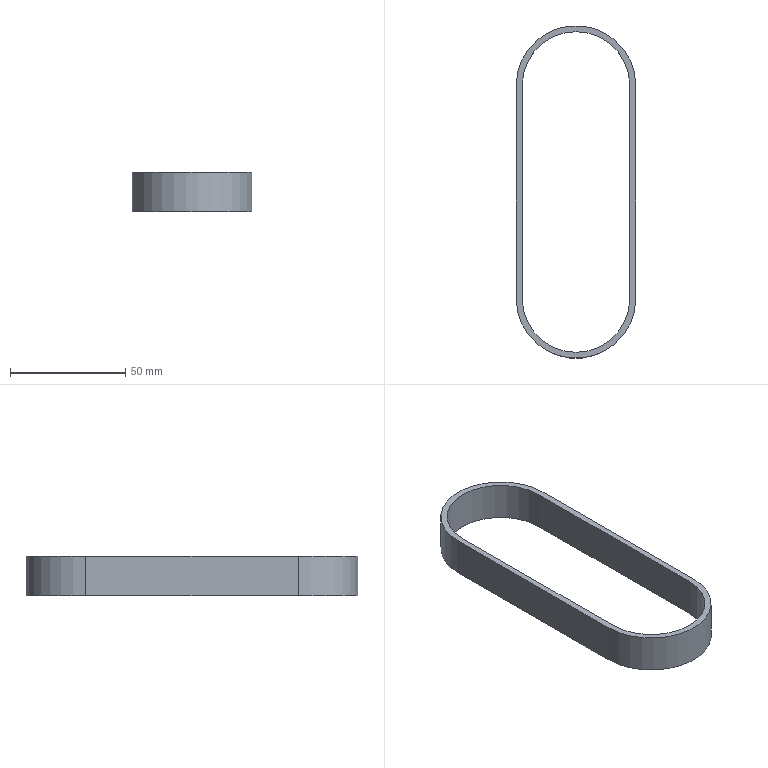Part | NX | features BREP 1 | 1 solid | 10 faces | box 52 x 144.5 x 17 mm | volume 15065 mm3 | plane 6 | cylinder 4 | commonest cylinder face diameters 46.79 x2 52 x2
STEP:
#1=CARTESIAN_POINT('',(54.,-107.5,-221.5));
#2=VERTEX_POINT('',#1);
#3=CARTESIAN_POINT('',(54.,-107.5,-204.5));
#4=VERTEX_POINT('',#3);
#5=CARTESIAN_POINT('',(54.,-107.5,-204.5));
#6=DIRECTION('',(0.,0.,1.));
#7=VECTOR('',#6,1000.);
#8=LINE('',#5,#7);
#9=EDGE_CURVE('',#2,#4,#8,.T.);
#10=ORIENTED_EDGE('',*,*,#9,.T.);
#11=CARTESIAN_POINT('',(54.,-15.,-204.5));
#12=VERTEX_POINT('',#11);
#13=CARTESIAN_POINT('',(54.,-107.5,-204.5));
#14=DIRECTION('',(0.,1.,0.));
#15=VECTOR('',#14,1000.);
#16=LINE('',#13,#15);
#17=EDGE_CURVE('',#4,#12,#16,.T.);
#18=ORIENTED_EDGE('',*,*,#17,.T.);
#19=CARTESIAN_POINT('',(54.,-15.,-221.5));
#20=VERTEX_POINT('',#19);
#21=CARTESIAN_POINT('',(54.,-15.,-204.5));
#22=DIRECTION('',(0.,0.,-1.));
#23=VECTOR('',#22,1000.);
#24=LINE('',#21,#23);
#25=EDGE_CURVE('',#12,#20,#24,.T.);
#26=ORIENTED_EDGE('',*,*,#25,.T.);
#27=CARTESIAN_POINT('',(54.,-107.5,-221.5));
#28=DIRECTION('',(0.,-1.,0.));
#29=VECTOR('',#28,1000.);
#30=LINE('',#27,#29);
#31=EDGE_CURVE('',#20,#2,#30,.T.);
#32=ORIENTED_EDGE('',*,*,#31,.T.);
#33=EDGE_LOOP('',(#10,#18,#26,#32));
#34=FACE_BOUND('',#33,.T.);
#35=CARTESIAN_POINT('',(54.,-107.5,-204.5));
#36=DIRECTION('',(-1.,0.,0.));
#37=DIRECTION('',(0.,0.,1.));
#38=AXIS2_PLACEMENT_3D('',#35,#36,#37);
#39=PLANE('',#38);
#40=ADVANCED_FACE('',(#34),#39,.T.);
#41=CARTESIAN_POINT('',(106.,-15.,-204.5));
#42=VERTEX_POINT('',#41);
#43=CARTESIAN_POINT('',(106.,-107.5,-204.5));
#44=VERTEX_POINT('',#43);
#45=CARTESIAN_POINT('',(106.,0.,-204.5));
#46=DIRECTION('',(0.,-1.,0.));
#47=VECTOR('',#46,1000.);
#48=LINE('',#45,#47);
#49=EDGE_CURVE('',#42,#44,#48,.T.);
#50=ORIENTED_EDGE('',*,*,#49,.F.);
#51=CARTESIAN_POINT('',(80.,-15.,-204.5));
#52=DIRECTION('',(0.,0.,-1.));
#53=DIRECTION('',(-1.,0.,0.));
#54=AXIS2_PLACEMENT_3D('',#51,#52,#53);
#55=CIRCLE('',#54,26.);
#56=EDGE_CURVE('',#12,#42,#55,.T.);
#57=ORIENTED_EDGE('',*,*,#56,.F.);
#58=ORIENTED_EDGE('',*,*,#17,.F.);
#59=CARTESIAN_POINT('',(80.,-107.5,-204.5));
#60=DIRECTION('',(0.,0.,-1.));
#61=DIRECTION('',(-1.,0.,0.));
#62=AXIS2_PLACEMENT_3D('',#59,#60,#61);
#63=CIRCLE('',#62,26.);
#64=EDGE_CURVE('',#44,#4,#63,.T.);
#65=ORIENTED_EDGE('',*,*,#64,.F.);
#66=EDGE_LOOP('',(#50,#57,#58,#65));
#67=FACE_BOUND('',#66,.T.);
#68=CARTESIAN_POINT('',(56.605,-15.,-204.5));
#69=VERTEX_POINT('',#68);
#70=CARTESIAN_POINT('',(56.605,-107.5,-204.5));
#71=VERTEX_POINT('',#70);
#72=CARTESIAN_POINT('',(56.605,0.,-204.5));
#73=DIRECTION('',(0.,-1.,0.));
#74=VECTOR('',#73,1000.);
#75=LINE('',#72,#74);
#76=EDGE_CURVE('',#69,#71,#75,.T.);
#77=ORIENTED_EDGE('',*,*,#76,.F.);
#78=CARTESIAN_POINT('',(103.395,-15.,-204.5));
#79=VERTEX_POINT('',#78);
#80=CARTESIAN_POINT('',(80.,-15.,-204.5));
#81=DIRECTION('',(0.,0.,1.));
#82=DIRECTION('',(-1.,0.,0.));
#83=AXIS2_PLACEMENT_3D('',#80,#81,#82);
#84=CIRCLE('',#83,23.395);
#85=EDGE_CURVE('',#79,#69,#84,.T.);
#86=ORIENTED_EDGE('',*,*,#85,.F.);
#87=CARTESIAN_POINT('',(103.395,-107.5,-204.5));
#88=VERTEX_POINT('',#87);
#89=CARTESIAN_POINT('',(103.395,0.,-204.5));
#90=DIRECTION('',(0.,1.,0.));
#91=VECTOR('',#90,1000.);
#92=LINE('',#89,#91);
#93=EDGE_CURVE('',#88,#79,#92,.T.);
#94=ORIENTED_EDGE('',*,*,#93,.F.);
#95=CARTESIAN_POINT('',(80.,-107.5,-204.5));
#96=DIRECTION('',(0.,0.,1.));
#97=DIRECTION('',(-1.,0.,0.));
#98=AXIS2_PLACEMENT_3D('',#95,#96,#97);
#99=CIRCLE('',#98,23.395);
#100=EDGE_CURVE('',#71,#88,#99,.T.);
#101=ORIENTED_EDGE('',*,*,#100,.F.);
#102=EDGE_LOOP('',(#77,#86,#94,#101));
#103=FACE_BOUND('',#102,.T.);
#104=CARTESIAN_POINT('',(0.,0.,-204.5));
#105=DIRECTION('',(0.,0.,-1.));
#106=DIRECTION('',(0.,-1.,0.));
#107=AXIS2_PLACEMENT_3D('',#104,#105,#106);
#108=PLANE('',#107);
#109=ADVANCED_FACE('',(#67,#103),#108,.F.);
#110=CARTESIAN_POINT('',(106.,-107.5,-221.5));
#111=VERTEX_POINT('',#110);
#112=CARTESIAN_POINT('',(106.,-107.5,-204.5));
#113=DIRECTION('',(0.,0.,1.));
#114=VECTOR('',#113,1000.);
#115=LINE('',#112,#114);
#116=EDGE_CURVE('',#111,#44,#115,.T.);
#117=ORIENTED_EDGE('',*,*,#116,.T.);
#118=ORIENTED_EDGE('',*,*,#64,.T.);
#119=ORIENTED_EDGE('',*,*,#9,.F.);
#120=CARTESIAN_POINT('',(80.,-107.5,-221.5));
#121=DIRECTION('',(0.,0.,1.));
#122=DIRECTION('',(-1.,0.,0.));
#123=AXIS2_PLACEMENT_3D('',#120,#121,#122);
#124=CIRCLE('',#123,26.);
#125=EDGE_CURVE('',#2,#111,#124,.T.);
#126=ORIENTED_EDGE('',*,*,#125,.T.);
#127=EDGE_LOOP('',(#117,#118,#119,#126));
#128=FACE_BOUND('',#127,.T.);
#129=CARTESIAN_POINT('',(80.,-107.5,-204.5));
#130=DIRECTION('',(0.,0.,-1.));
#131=DIRECTION('',(-1.,0.,0.));
#132=AXIS2_PLACEMENT_3D('',#129,#130,#131);
#133=CYLINDRICAL_SURFACE('',#132,26.);
#134=ADVANCED_FACE('',(#128),#133,.T.);
#135=ORIENTED_EDGE('',*,*,#125,.F.);
#136=ORIENTED_EDGE('',*,*,#31,.F.);
#137=CARTESIAN_POINT('',(106.,-15.,-221.5));
#138=VERTEX_POINT('',#137);
#139=CARTESIAN_POINT('',(80.,-15.,-221.5));
#140=DIRECTION('',(0.,0.,-1.));
#141=DIRECTION('',(-1.,0.,0.));
#142=AXIS2_PLACEMENT_3D('',#139,#140,#141);
#143=CIRCLE('',#142,26.);
#144=EDGE_CURVE('',#20,#138,#143,.T.);
#145=ORIENTED_EDGE('',*,*,#144,.T.);
#146=CARTESIAN_POINT('',(106.,0.,-221.5));
#147=DIRECTION('',(0.,-1.,0.));
#148=VECTOR('',#147,1000.);
#149=LINE('',#146,#148);
#150=EDGE_CURVE('',#138,#111,#149,.T.);
#151=ORIENTED_EDGE('',*,*,#150,.T.);
#152=EDGE_LOOP('',(#135,#136,#145,#151));
#153=FACE_BOUND('',#152,.T.);
#154=CARTESIAN_POINT('',(56.605,-107.5,-221.5));
#155=VERTEX_POINT('',#154);
#156=CARTESIAN_POINT('',(103.395,-107.5,-221.5));
#157=VERTEX_POINT('',#156);
#158=CARTESIAN_POINT('',(80.,-107.5,-221.5));
#159=DIRECTION('',(0.,0.,1.));
#160=DIRECTION('',(-1.,0.,0.));
#161=AXIS2_PLACEMENT_3D('',#158,#159,#160);
#162=CIRCLE('',#161,23.395);
#163=EDGE_CURVE('',#155,#157,#162,.T.);
#164=ORIENTED_EDGE('',*,*,#163,.T.);
#165=CARTESIAN_POINT('',(103.395,-15.,-221.5));
#166=VERTEX_POINT('',#165);
#167=CARTESIAN_POINT('',(103.395,0.,-221.5));
#168=DIRECTION('',(0.,1.,0.));
#169=VECTOR('',#168,1000.);
#170=LINE('',#167,#169);
#171=EDGE_CURVE('',#157,#166,#170,.T.);
#172=ORIENTED_EDGE('',*,*,#171,.T.);
#173=CARTESIAN_POINT('',(56.605,-15.,-221.5));
#174=VERTEX_POINT('',#173);
#175=CARTESIAN_POINT('',(80.,-15.,-221.5));
#176=DIRECTION('',(0.,0.,1.));
#177=DIRECTION('',(-1.,0.,0.));
#178=AXIS2_PLACEMENT_3D('',#175,#176,#177);
#179=CIRCLE('',#178,23.395);
#180=EDGE_CURVE('',#166,#174,#179,.T.);
#181=ORIENTED_EDGE('',*,*,#180,.T.);
#182=CARTESIAN_POINT('',(56.605,0.,-221.5));
#183=DIRECTION('',(0.,-1.,0.));
#184=VECTOR('',#183,1000.);
#185=LINE('',#182,#184);
#186=EDGE_CURVE('',#174,#155,#185,.T.);
#187=ORIENTED_EDGE('',*,*,#186,.T.);
#188=EDGE_LOOP('',(#164,#172,#181,#187));
#189=FACE_BOUND('',#188,.T.);
#190=CARTESIAN_POINT('',(0.,0.,-221.5));
#191=DIRECTION('',(0.,0.,-1.));
#192=DIRECTION('',(0.,-1.,0.));
#193=AXIS2_PLACEMENT_3D('',#190,#191,#192);
#194=PLANE('',#193);
#195=ADVANCED_FACE('',(#153,#189),#194,.T.);
#196=ORIENTED_EDGE('',*,*,#25,.F.);
#197=ORIENTED_EDGE('',*,*,#56,.T.);
#198=CARTESIAN_POINT('',(106.,-15.,-204.5));
#199=DIRECTION('',(0.,0.,-1.));
#200=VECTOR('',#199,1000.);
#201=LINE('',#198,#200);
#202=EDGE_CURVE('',#42,#138,#201,.T.);
#203=ORIENTED_EDGE('',*,*,#202,.T.);
#204=ORIENTED_EDGE('',*,*,#144,.F.);
#205=EDGE_LOOP('',(#196,#197,#203,#204));
#206=FACE_BOUND('',#205,.T.);
#207=CARTESIAN_POINT('',(80.,-15.,-204.5));
#208=DIRECTION('',(0.,0.,-1.));
#209=DIRECTION('',(-1.,0.,0.));
#210=AXIS2_PLACEMENT_3D('',#207,#208,#209);
#211=CYLINDRICAL_SURFACE('',#210,26.);
#212=ADVANCED_FACE('',(#206),#211,.T.);
#213=ORIENTED_EDGE('',*,*,#163,.F.);
#214=CARTESIAN_POINT('',(56.605,-107.5,-204.5));
#215=DIRECTION('',(0.,0.,-1.));
#216=VECTOR('',#215,1000.);
#217=LINE('',#214,#216);
#218=EDGE_CURVE('',#71,#155,#217,.T.);
#219=ORIENTED_EDGE('',*,*,#218,.F.);
#220=ORIENTED_EDGE('',*,*,#100,.T.);
#221=CARTESIAN_POINT('',(103.395,-107.5,-204.5));
#222=DIRECTION('',(0.,0.,1.));
#223=VECTOR('',#222,1000.);
#224=LINE('',#221,#223);
#225=EDGE_CURVE('',#157,#88,#224,.T.);
#226=ORIENTED_EDGE('',*,*,#225,.F.);
#227=EDGE_LOOP('',(#213,#219,#220,#226));
#228=FACE_BOUND('',#227,.T.);
#229=CARTESIAN_POINT('',(80.,-107.5,-204.5));
#230=DIRECTION('',(0.,0.,-1.));
#231=DIRECTION('',(-1.,0.,0.));
#232=AXIS2_PLACEMENT_3D('',#229,#230,#231);
#233=CYLINDRICAL_SURFACE('',#232,23.395);
#234=ADVANCED_FACE('',(#228),#233,.F.);
#235=CARTESIAN_POINT('',(56.605,-15.,-204.5));
#236=DIRECTION('',(0.,0.,1.));
#237=VECTOR('',#236,1000.);
#238=LINE('',#235,#237);
#239=EDGE_CURVE('',#174,#69,#238,.T.);
#240=ORIENTED_EDGE('',*,*,#239,.T.);
#241=ORIENTED_EDGE('',*,*,#76,.T.);
#242=ORIENTED_EDGE('',*,*,#218,.T.);
#243=ORIENTED_EDGE('',*,*,#186,.F.);
#244=EDGE_LOOP('',(#240,#241,#242,#243));
#245=FACE_BOUND('',#244,.T.);
#246=CARTESIAN_POINT('',(56.605,-15.,-204.5));
#247=DIRECTION('',(1.,0.,0.));
#248=DIRECTION('',(0.,1.,0.));
#249=AXIS2_PLACEMENT_3D('',#246,#247,#248);
#250=PLANE('',#249);
#251=ADVANCED_FACE('',(#245),#250,.T.);
#252=ORIENTED_EDGE('',*,*,#180,.F.);
#253=CARTESIAN_POINT('',(103.395,-15.,-204.5));
#254=DIRECTION('',(0.,0.,-1.));
#255=VECTOR('',#254,1000.);
#256=LINE('',#253,#255);
#257=EDGE_CURVE('',#79,#166,#256,.T.);
#258=ORIENTED_EDGE('',*,*,#257,.F.);
#259=ORIENTED_EDGE('',*,*,#85,.T.);
#260=ORIENTED_EDGE('',*,*,#239,.F.);
#261=EDGE_LOOP('',(#252,#258,#259,#260));
#262=FACE_BOUND('',#261,.T.);
#263=CARTESIAN_POINT('',(80.,-15.,-204.5));
#264=DIRECTION('',(0.,0.,-1.));
#265=DIRECTION('',(-1.,0.,0.));
#266=AXIS2_PLACEMENT_3D('',#263,#264,#265);
#267=CYLINDRICAL_SURFACE('',#266,23.395);
#268=ADVANCED_FACE('',(#262),#267,.F.);
#269=ORIENTED_EDGE('',*,*,#225,.T.);
#270=ORIENTED_EDGE('',*,*,#93,.T.);
#271=ORIENTED_EDGE('',*,*,#257,.T.);
#272=ORIENTED_EDGE('',*,*,#171,.F.);
#273=EDGE_LOOP('',(#269,#270,#271,#272));
#274=FACE_BOUND('',#273,.T.);
#275=CARTESIAN_POINT('',(103.395,-107.5,-204.5));
#276=DIRECTION('',(-1.,0.,0.));
#277=DIRECTION('',(0.,0.,1.));
#278=AXIS2_PLACEMENT_3D('',#275,#276,#277);
#279=PLANE('',#278);
#280=ADVANCED_FACE('',(#274),#279,.T.);
#281=ORIENTED_EDGE('',*,*,#202,.F.);
#282=ORIENTED_EDGE('',*,*,#49,.T.);
#283=ORIENTED_EDGE('',*,*,#116,.F.);
#284=ORIENTED_EDGE('',*,*,#150,.F.);
#285=EDGE_LOOP('',(#281,#282,#283,#284));
#286=FACE_BOUND('',#285,.T.);
#287=CARTESIAN_POINT('',(106.,-15.,-204.5));
#288=DIRECTION('',(1.,0.,0.));
#289=DIRECTION('',(0.,1.,0.));
#290=AXIS2_PLACEMENT_3D('',#287,#288,#289);
#291=PLANE('',#290);
#292=ADVANCED_FACE('',(#286),#291,.T.);
#293=CLOSED_SHELL('',(#40,#109,#134,#195,#212,#234,#251,#268,#280,#292));
#294=MANIFOLD_SOLID_BREP('',#293);
#295=(LENGTH_UNIT()NAMED_UNIT(*)SI_UNIT(.MILLI.,.METRE.));
#296=UNCERTAINTY_MEASURE_WITH_UNIT(LENGTH_MEASURE(0.00001),#295,'','');
#297=(NAMED_UNIT(*)PLANE_ANGLE_UNIT()SI_UNIT($,.RADIAN.));
#298=(NAMED_UNIT(*)SI_UNIT($,.STERADIAN.)SOLID_ANGLE_UNIT());
#299=(GEOMETRIC_REPRESENTATION_CONTEXT(3)GLOBAL_UNCERTAINTY_ASSIGNED_CONTEXT((#296))GLOBAL_UNIT_ASSIGNED_CONTEXT((#295,#297,#298))REPRESENTATION_CONTEXT('',''));
#300=ADVANCED_BREP_SHAPE_REPRESENTATION('',(#294),#299);